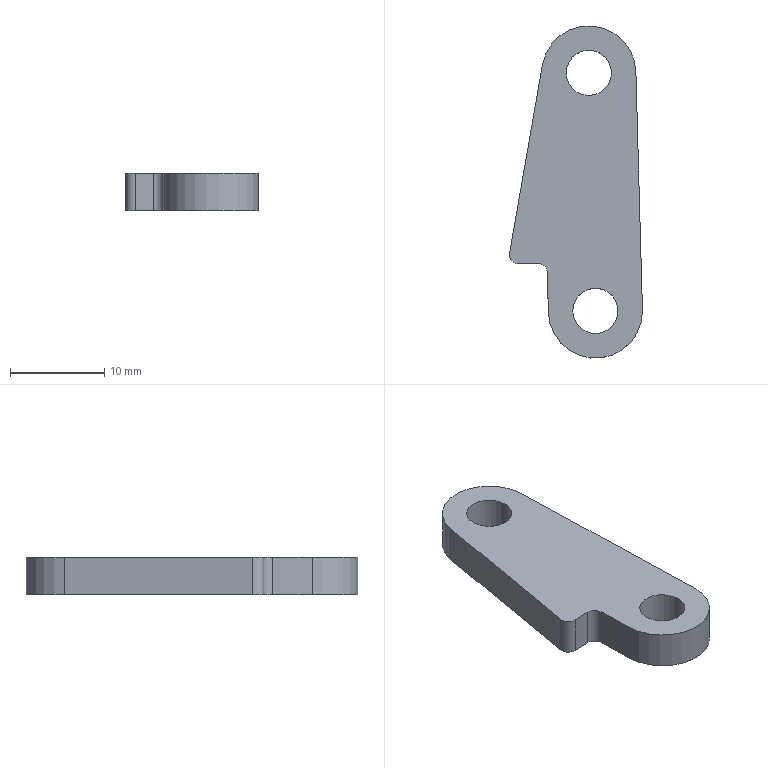Part | SolidWorks | features BaseBody 1 | 1 solid | 15 faces | box 14.127 x 35.318 x 4 mm | volume 1354 mm3 | cylinder 9 | plane 6 | commonest cylinder face diameters 4.8 x4 10 x3 2 x2
STEP:
#1=CARTESIAN_POINT('',(-4.999,-0.1072,-2.));
#2=VERTEX_POINT('',#1);
#3=CARTESIAN_POINT('',(5.,0.,-2.));
#4=VERTEX_POINT('',#3);
#5=CARTESIAN_POINT('',(0.,0.,-2.));
#6=DIRECTION('',(0.,0.,1.));
#7=DIRECTION('',(1.,0.,0.));
#8=AXIS2_PLACEMENT_3D('',#5,#6,#7);
#9=CIRCLE('',#8,5.);
#10=EDGE_CURVE('',#2,#4,#9,.T.);
#11=ORIENTED_EDGE('',*,*,#10,.T.);
#12=CARTESIAN_POINT('',(5.,0.,2.));
#13=VERTEX_POINT('',#12);
#14=CARTESIAN_POINT('',(5.,0.,2.));
#15=DIRECTION('',(0.,0.,1.));
#16=VECTOR('',#15,1000.);
#17=LINE('',#14,#16);
#18=EDGE_CURVE('',#4,#13,#17,.T.);
#19=ORIENTED_EDGE('',*,*,#18,.T.);
#20=CARTESIAN_POINT('',(-4.999,-0.1072,2.));
#21=VERTEX_POINT('',#20);
#22=CARTESIAN_POINT('',(0.,0.,2.));
#23=DIRECTION('',(0.,0.,1.));
#24=DIRECTION('',(1.,0.,0.));
#25=AXIS2_PLACEMENT_3D('',#22,#23,#24);
#26=CIRCLE('',#25,5.);
#27=EDGE_CURVE('',#21,#13,#26,.T.);
#28=ORIENTED_EDGE('',*,*,#27,.F.);
#29=CARTESIAN_POINT('',(-4.999,-0.1072,2.));
#30=DIRECTION('',(0.,0.,-1.));
#31=VECTOR('',#30,1000.);
#32=LINE('',#29,#31);
#33=EDGE_CURVE('',#21,#2,#32,.T.);
#34=ORIENTED_EDGE('',*,*,#33,.T.);
#35=EDGE_LOOP('',(#11,#19,#28,#34));
#36=FACE_OUTER_BOUND('',#35,.T.);
#37=CARTESIAN_POINT('',(0.,0.,2.));
#38=DIRECTION('',(0.,0.,1.));
#39=DIRECTION('',(1.,0.,0.));
#40=AXIS2_PLACEMENT_3D('',#37,#38,#39);
#41=CYLINDRICAL_SURFACE('',#40,5.);
#42=ADVANCED_FACE('',(#36),#41,.T.);
#43=CARTESIAN_POINT('',(-2.401,0.03084,-2.));
#44=VERTEX_POINT('',#43);
#45=CARTESIAN_POINT('',(2.399,0.03084,-2.));
#46=VERTEX_POINT('',#45);
#47=CARTESIAN_POINT('',(-0.0008516,0.03084,-2.));
#48=DIRECTION('',(0.,0.,1.));
#49=DIRECTION('',(1.,0.,0.));
#50=AXIS2_PLACEMENT_3D('',#47,#48,#49);
#51=CIRCLE('',#50,2.4);
#52=EDGE_CURVE('',#44,#46,#51,.T.);
#53=ORIENTED_EDGE('',*,*,#52,.F.);
#54=CARTESIAN_POINT('',(-2.401,0.03084,2.));
#55=VERTEX_POINT('',#54);
#56=CARTESIAN_POINT('',(-2.401,0.03084,2.));
#57=DIRECTION('',(0.,0.,1.));
#58=VECTOR('',#57,1000.);
#59=LINE('',#56,#58);
#60=EDGE_CURVE('',#44,#55,#59,.T.);
#61=ORIENTED_EDGE('',*,*,#60,.T.);
#62=CARTESIAN_POINT('',(2.399,0.03084,2.));
#63=VERTEX_POINT('',#62);
#64=CARTESIAN_POINT('',(-0.0008516,0.03084,2.));
#65=DIRECTION('',(0.,0.,-1.));
#66=DIRECTION('',(1.,0.,0.));
#67=AXIS2_PLACEMENT_3D('',#64,#65,#66);
#68=CIRCLE('',#67,2.4);
#69=EDGE_CURVE('',#63,#55,#68,.T.);
#70=ORIENTED_EDGE('',*,*,#69,.F.);
#71=CARTESIAN_POINT('',(2.399,0.03084,2.));
#72=DIRECTION('',(0.,0.,1.));
#73=VECTOR('',#72,1000.);
#74=LINE('',#71,#73);
#75=EDGE_CURVE('',#46,#63,#74,.T.);
#76=ORIENTED_EDGE('',*,*,#75,.F.);
#77=EDGE_LOOP('',(#53,#61,#70,#76));
#78=FACE_OUTER_BOUND('',#77,.T.);
#79=CARTESIAN_POINT('',(-0.0008516,0.03084,2.));
#80=DIRECTION('',(0.,0.,1.));
#81=DIRECTION('',(1.,0.,0.));
#82=AXIS2_PLACEMENT_3D('',#79,#80,#81);
#83=CYLINDRICAL_SURFACE('',#82,2.4);
#84=ADVANCED_FACE('',(#78),#83,.F.);
#85=CARTESIAN_POINT('',(-3.101,25.331,-2.));
#86=VERTEX_POINT('',#85);
#87=CARTESIAN_POINT('',(1.699,25.331,-2.));
#88=VERTEX_POINT('',#87);
#89=CARTESIAN_POINT('',(-0.7009,25.331,-2.));
#90=DIRECTION('',(0.,0.,1.));
#91=DIRECTION('',(1.,0.,0.));
#92=AXIS2_PLACEMENT_3D('',#89,#90,#91);
#93=CIRCLE('',#92,2.4);
#94=EDGE_CURVE('',#86,#88,#93,.T.);
#95=ORIENTED_EDGE('',*,*,#94,.F.);
#96=CARTESIAN_POINT('',(-3.101,25.331,2.));
#97=VERTEX_POINT('',#96);
#98=CARTESIAN_POINT('',(-3.101,25.331,2.));
#99=DIRECTION('',(0.,0.,1.));
#100=VECTOR('',#99,1000.);
#101=LINE('',#98,#100);
#102=EDGE_CURVE('',#86,#97,#101,.T.);
#103=ORIENTED_EDGE('',*,*,#102,.T.);
#104=CARTESIAN_POINT('',(1.699,25.331,2.));
#105=VERTEX_POINT('',#104);
#106=CARTESIAN_POINT('',(-0.7009,25.331,2.));
#107=DIRECTION('',(0.,0.,-1.));
#108=DIRECTION('',(1.,0.,0.));
#109=AXIS2_PLACEMENT_3D('',#106,#107,#108);
#110=CIRCLE('',#109,2.4);
#111=EDGE_CURVE('',#105,#97,#110,.T.);
#112=ORIENTED_EDGE('',*,*,#111,.F.);
#113=CARTESIAN_POINT('',(1.699,25.331,2.));
#114=DIRECTION('',(0.,0.,1.));
#115=VECTOR('',#114,1000.);
#116=LINE('',#113,#115);
#117=EDGE_CURVE('',#88,#105,#116,.T.);
#118=ORIENTED_EDGE('',*,*,#117,.F.);
#119=EDGE_LOOP('',(#95,#103,#112,#118));
#120=FACE_OUTER_BOUND('',#119,.T.);
#121=CARTESIAN_POINT('',(-0.7009,25.331,2.));
#122=DIRECTION('',(0.,0.,1.));
#123=DIRECTION('',(1.,0.,0.));
#124=AXIS2_PLACEMENT_3D('',#121,#122,#123);
#125=CYLINDRICAL_SURFACE('',#124,2.4);
#126=ADVANCED_FACE('',(#120),#125,.F.);
#127=CARTESIAN_POINT('',(4.997,0.1688,2.));
#128=VERTEX_POINT('',#127);
#129=CARTESIAN_POINT('',(4.299,25.459,2.));
#130=VERTEX_POINT('',#129);
#131=CARTESIAN_POINT('',(4.997,0.1688,2.));
#132=DIRECTION('',(-0.02759,0.9996,0.));
#133=VECTOR('',#132,1000.);
#134=LINE('',#131,#133);
#135=EDGE_CURVE('',#128,#130,#134,.T.);
#136=ORIENTED_EDGE('',*,*,#135,.T.);
#137=CARTESIAN_POINT('',(-5.624,26.181,2.));
#138=VERTEX_POINT('',#137);
#139=CARTESIAN_POINT('',(-0.6989,25.318,2.));
#140=DIRECTION('',(0.,0.,1.));
#141=DIRECTION('',(1.,0.,0.));
#142=AXIS2_PLACEMENT_3D('',#139,#140,#141);
#143=CIRCLE('',#142,5.);
#144=EDGE_CURVE('',#130,#138,#143,.T.);
#145=ORIENTED_EDGE('',*,*,#144,.T.);
#146=CARTESIAN_POINT('',(-9.112,6.191,2.));
#147=VERTEX_POINT('',#146);
#148=CARTESIAN_POINT('',(-5.624,26.181,2.));
#149=DIRECTION('',(-0.1719,-0.9851,0.));
#150=VECTOR('',#149,1000.);
#151=LINE('',#148,#150);
#152=EDGE_CURVE('',#138,#147,#151,.T.);
#153=ORIENTED_EDGE('',*,*,#152,.T.);
#154=CARTESIAN_POINT('',(-8.099,5.02,2.));
#155=VERTEX_POINT('',#154);
#156=CARTESIAN_POINT('',(-8.127,6.019,2.));
#157=DIRECTION('',(0.,0.,1.));
#158=DIRECTION('',(1.,0.,0.));
#159=AXIS2_PLACEMENT_3D('',#156,#157,#158);
#160=CIRCLE('',#159,1.);
#161=EDGE_CURVE('',#147,#155,#160,.T.);
#162=ORIENTED_EDGE('',*,*,#161,.T.);
#163=CARTESIAN_POINT('',(-6.142,5.074,2.));
#164=VERTEX_POINT('',#163);
#165=CARTESIAN_POINT('',(-8.099,5.02,2.));
#166=DIRECTION('',(0.9996,0.0276,0.));
#167=VECTOR('',#166,1000.);
#168=LINE('',#165,#167);
#169=EDGE_CURVE('',#155,#164,#168,.T.);
#170=ORIENTED_EDGE('',*,*,#169,.T.);
#171=CARTESIAN_POINT('',(-5.115,4.102,2.));
#172=VERTEX_POINT('',#171);
#173=CARTESIAN_POINT('',(-6.114,4.074,2.));
#174=DIRECTION('',(0.,0.,-1.));
#175=DIRECTION('',(1.,0.,0.));
#176=AXIS2_PLACEMENT_3D('',#173,#174,#175);
#177=CIRCLE('',#176,1.);
#178=EDGE_CURVE('',#164,#172,#177,.T.);
#179=ORIENTED_EDGE('',*,*,#178,.T.);
#180=CARTESIAN_POINT('',(-5.115,4.102,2.));
#181=DIRECTION('',(0.02755,-0.9996,0.));
#182=VECTOR('',#181,1000.);
#183=LINE('',#180,#182);
#184=EDGE_CURVE('',#172,#21,#183,.T.);
#185=ORIENTED_EDGE('',*,*,#184,.T.);
#186=ORIENTED_EDGE('',*,*,#27,.T.);
#187=CARTESIAN_POINT('',(0.,0.,2.));
#188=DIRECTION('',(0.,0.,1.));
#189=DIRECTION('',(1.,0.,0.));
#190=AXIS2_PLACEMENT_3D('',#187,#188,#189);
#191=CIRCLE('',#190,5.);
#192=EDGE_CURVE('',#13,#128,#191,.T.);
#193=ORIENTED_EDGE('',*,*,#192,.T.);
#194=EDGE_LOOP('',(#136,#145,#153,#162,#170,#179,#185,#186,#193));
#195=FACE_OUTER_BOUND('',#194,.T.);
#196=ORIENTED_EDGE('',*,*,#69,.T.);
#197=CARTESIAN_POINT('',(-0.0008516,0.03084,2.));
#198=DIRECTION('',(0.,0.,-1.));
#199=DIRECTION('',(1.,0.,0.));
#200=AXIS2_PLACEMENT_3D('',#197,#198,#199);
#201=CIRCLE('',#200,2.4);
#202=EDGE_CURVE('',#55,#63,#201,.T.);
#203=ORIENTED_EDGE('',*,*,#202,.T.);
#204=EDGE_LOOP('',(#196,#203));
#205=FACE_BOUND('',#204,.T.);
#206=ORIENTED_EDGE('',*,*,#111,.T.);
#207=CARTESIAN_POINT('',(-0.7009,25.331,2.));
#208=DIRECTION('',(0.,0.,-1.));
#209=DIRECTION('',(1.,0.,0.));
#210=AXIS2_PLACEMENT_3D('',#207,#208,#209);
#211=CIRCLE('',#210,2.4);
#212=EDGE_CURVE('',#97,#105,#211,.T.);
#213=ORIENTED_EDGE('',*,*,#212,.T.);
#214=EDGE_LOOP('',(#206,#213));
#215=FACE_BOUND('',#214,.T.);
#216=CARTESIAN_POINT('',(-8.127,6.019,2.));
#217=DIRECTION('',(0.,0.,1.));
#218=DIRECTION('',(1.,0.,0.));
#219=AXIS2_PLACEMENT_3D('',#216,#217,#218);
#220=PLANE('',#219);
#221=ADVANCED_FACE('',(#195,#205,#215),#220,.T.);
#222=ORIENTED_EDGE('',*,*,#144,.F.);
#223=CARTESIAN_POINT('',(4.299,25.459,-2.));
#224=VERTEX_POINT('',#223);
#225=CARTESIAN_POINT('',(4.299,25.459,2.));
#226=DIRECTION('',(0.,0.,-1.));
#227=VECTOR('',#226,1000.);
#228=LINE('',#225,#227);
#229=EDGE_CURVE('',#130,#224,#228,.T.);
#230=ORIENTED_EDGE('',*,*,#229,.T.);
#231=CARTESIAN_POINT('',(-5.624,26.181,-2.));
#232=VERTEX_POINT('',#231);
#233=CARTESIAN_POINT('',(-0.6989,25.318,-2.));
#234=DIRECTION('',(0.,0.,1.));
#235=DIRECTION('',(1.,0.,0.));
#236=AXIS2_PLACEMENT_3D('',#233,#234,#235);
#237=CIRCLE('',#236,5.);
#238=EDGE_CURVE('',#224,#232,#237,.T.);
#239=ORIENTED_EDGE('',*,*,#238,.T.);
#240=CARTESIAN_POINT('',(-5.624,26.181,2.));
#241=DIRECTION('',(0.,0.,1.));
#242=VECTOR('',#241,1000.);
#243=LINE('',#240,#242);
#244=EDGE_CURVE('',#232,#138,#243,.T.);
#245=ORIENTED_EDGE('',*,*,#244,.T.);
#246=EDGE_LOOP('',(#222,#230,#239,#245));
#247=FACE_OUTER_BOUND('',#246,.T.);
#248=CARTESIAN_POINT('',(-0.6989,25.318,2.));
#249=DIRECTION('',(0.,0.,1.));
#250=DIRECTION('',(1.,0.,0.));
#251=AXIS2_PLACEMENT_3D('',#248,#249,#250);
#252=CYLINDRICAL_SURFACE('',#251,5.);
#253=ADVANCED_FACE('',(#247),#252,.T.);
#254=ORIENTED_EDGE('',*,*,#229,.F.);
#255=ORIENTED_EDGE('',*,*,#135,.F.);
#256=CARTESIAN_POINT('',(4.997,0.1688,-2.));
#257=VERTEX_POINT('',#256);
#258=CARTESIAN_POINT('',(4.997,0.1688,2.));
#259=DIRECTION('',(0.,0.,1.));
#260=VECTOR('',#259,1000.);
#261=LINE('',#258,#260);
#262=EDGE_CURVE('',#257,#128,#261,.T.);
#263=ORIENTED_EDGE('',*,*,#262,.F.);
#264=CARTESIAN_POINT('',(4.997,0.1688,-2.));
#265=DIRECTION('',(0.02759,-0.9996,0.));
#266=VECTOR('',#265,1000.);
#267=LINE('',#264,#266);
#268=EDGE_CURVE('',#224,#257,#267,.T.);
#269=ORIENTED_EDGE('',*,*,#268,.F.);
#270=EDGE_LOOP('',(#254,#255,#263,#269));
#271=FACE_OUTER_BOUND('',#270,.T.);
#272=CARTESIAN_POINT('',(4.997,0.1688,2.));
#273=DIRECTION('',(-0.9996,-0.02759,0.));
#274=DIRECTION('',(0.02759,-0.9996,0.));
#275=AXIS2_PLACEMENT_3D('',#272,#273,#274);
#276=PLANE('',#275);
#277=ADVANCED_FACE('',(#271),#276,.F.);
#278=ORIENTED_EDGE('',*,*,#18,.F.);
#279=CARTESIAN_POINT('',(0.,0.,-2.));
#280=DIRECTION('',(0.,0.,1.));
#281=DIRECTION('',(1.,0.,0.));
#282=AXIS2_PLACEMENT_3D('',#279,#280,#281);
#283=CIRCLE('',#282,5.);
#284=EDGE_CURVE('',#4,#257,#283,.T.);
#285=ORIENTED_EDGE('',*,*,#284,.T.);
#286=ORIENTED_EDGE('',*,*,#262,.T.);
#287=ORIENTED_EDGE('',*,*,#192,.F.);
#288=EDGE_LOOP('',(#278,#285,#286,#287));
#289=FACE_OUTER_BOUND('',#288,.T.);
#290=CARTESIAN_POINT('',(0.,0.,2.));
#291=DIRECTION('',(0.,0.,1.));
#292=DIRECTION('',(1.,0.,0.));
#293=AXIS2_PLACEMENT_3D('',#290,#291,#292);
#294=CYLINDRICAL_SURFACE('',#293,5.);
#295=ADVANCED_FACE('',(#289),#294,.T.);
#296=ORIENTED_EDGE('',*,*,#33,.F.);
#297=ORIENTED_EDGE('',*,*,#184,.F.);
#298=CARTESIAN_POINT('',(-5.115,4.102,-2.));
#299=VERTEX_POINT('',#298);
#300=CARTESIAN_POINT('',(-5.115,4.102,2.));
#301=DIRECTION('',(0.,0.,1.));
#302=VECTOR('',#301,1000.);
#303=LINE('',#300,#302);
#304=EDGE_CURVE('',#299,#172,#303,.T.);
#305=ORIENTED_EDGE('',*,*,#304,.F.);
#306=CARTESIAN_POINT('',(-5.115,4.102,-2.));
#307=DIRECTION('',(-0.02755,0.9996,0.));
#308=VECTOR('',#307,1000.);
#309=LINE('',#306,#308);
#310=EDGE_CURVE('',#2,#299,#309,.T.);
#311=ORIENTED_EDGE('',*,*,#310,.F.);
#312=EDGE_LOOP('',(#296,#297,#305,#311));
#313=FACE_OUTER_BOUND('',#312,.T.);
#314=CARTESIAN_POINT('',(-5.115,4.102,2.));
#315=DIRECTION('',(0.9996,0.02755,0.));
#316=DIRECTION('',(-0.02755,0.9996,0.));
#317=AXIS2_PLACEMENT_3D('',#314,#315,#316);
#318=PLANE('',#317);
#319=ADVANCED_FACE('',(#313),#318,.F.);
#320=CARTESIAN_POINT('',(-6.142,5.074,-2.));
#321=VERTEX_POINT('',#320);
#322=CARTESIAN_POINT('',(-6.142,5.074,2.));
#323=DIRECTION('',(0.,0.,-1.));
#324=VECTOR('',#323,1000.);
#325=LINE('',#322,#324);
#326=EDGE_CURVE('',#164,#321,#325,.T.);
#327=ORIENTED_EDGE('',*,*,#326,.F.);
#328=ORIENTED_EDGE('',*,*,#169,.F.);
#329=CARTESIAN_POINT('',(-8.099,5.02,-2.));
#330=VERTEX_POINT('',#329);
#331=CARTESIAN_POINT('',(-8.099,5.02,2.));
#332=DIRECTION('',(0.,0.,1.));
#333=VECTOR('',#332,1000.);
#334=LINE('',#331,#333);
#335=EDGE_CURVE('',#330,#155,#334,.T.);
#336=ORIENTED_EDGE('',*,*,#335,.F.);
#337=CARTESIAN_POINT('',(-8.099,5.02,-2.));
#338=DIRECTION('',(-0.9996,-0.0276,0.));
#339=VECTOR('',#338,1000.);
#340=LINE('',#337,#339);
#341=EDGE_CURVE('',#321,#330,#340,.T.);
#342=ORIENTED_EDGE('',*,*,#341,.F.);
#343=EDGE_LOOP('',(#327,#328,#336,#342));
#344=FACE_OUTER_BOUND('',#343,.T.);
#345=CARTESIAN_POINT('',(-8.099,5.02,2.));
#346=DIRECTION('',(-0.0276,0.9996,0.));
#347=DIRECTION('',(-0.9996,-0.0276,0.));
#348=AXIS2_PLACEMENT_3D('',#345,#346,#347);
#349=PLANE('',#348);
#350=ADVANCED_FACE('',(#344),#349,.F.);
#351=ORIENTED_EDGE('',*,*,#161,.F.);
#352=CARTESIAN_POINT('',(-9.112,6.191,-2.));
#353=VERTEX_POINT('',#352);
#354=CARTESIAN_POINT('',(-9.112,6.191,2.));
#355=DIRECTION('',(0.,0.,-1.));
#356=VECTOR('',#355,1000.);
#357=LINE('',#354,#356);
#358=EDGE_CURVE('',#147,#353,#357,.T.);
#359=ORIENTED_EDGE('',*,*,#358,.T.);
#360=CARTESIAN_POINT('',(-8.127,6.019,-2.));
#361=DIRECTION('',(0.,0.,1.));
#362=DIRECTION('',(1.,0.,0.));
#363=AXIS2_PLACEMENT_3D('',#360,#361,#362);
#364=CIRCLE('',#363,1.);
#365=EDGE_CURVE('',#353,#330,#364,.T.);
#366=ORIENTED_EDGE('',*,*,#365,.T.);
#367=ORIENTED_EDGE('',*,*,#335,.T.);
#368=EDGE_LOOP('',(#351,#359,#366,#367));
#369=FACE_OUTER_BOUND('',#368,.T.);
#370=CARTESIAN_POINT('',(-8.127,6.019,2.));
#371=DIRECTION('',(0.,0.,1.));
#372=DIRECTION('',(1.,0.,0.));
#373=AXIS2_PLACEMENT_3D('',#370,#371,#372);
#374=CYLINDRICAL_SURFACE('',#373,1.);
#375=ADVANCED_FACE('',(#369),#374,.T.);
#376=ORIENTED_EDGE('',*,*,#358,.F.);
#377=ORIENTED_EDGE('',*,*,#152,.F.);
#378=ORIENTED_EDGE('',*,*,#244,.F.);
#379=CARTESIAN_POINT('',(-5.624,26.181,-2.));
#380=DIRECTION('',(0.1719,0.9851,0.));
#381=VECTOR('',#380,1000.);
#382=LINE('',#379,#381);
#383=EDGE_CURVE('',#353,#232,#382,.T.);
#384=ORIENTED_EDGE('',*,*,#383,.F.);
#385=EDGE_LOOP('',(#376,#377,#378,#384));
#386=FACE_OUTER_BOUND('',#385,.T.);
#387=CARTESIAN_POINT('',(-5.624,26.181,2.));
#388=DIRECTION('',(0.9851,-0.1719,0.));
#389=DIRECTION('',(0.1719,0.9851,0.));
#390=AXIS2_PLACEMENT_3D('',#387,#388,#389);
#391=PLANE('',#390);
#392=ADVANCED_FACE('',(#386),#391,.F.);
#393=ORIENTED_EDGE('',*,*,#60,.F.);
#394=CARTESIAN_POINT('',(-0.0008516,0.03084,-2.));
#395=DIRECTION('',(0.,0.,1.));
#396=DIRECTION('',(1.,0.,0.));
#397=AXIS2_PLACEMENT_3D('',#394,#395,#396);
#398=CIRCLE('',#397,2.4);
#399=EDGE_CURVE('',#46,#44,#398,.T.);
#400=ORIENTED_EDGE('',*,*,#399,.F.);
#401=ORIENTED_EDGE('',*,*,#75,.T.);
#402=ORIENTED_EDGE('',*,*,#202,.F.);
#403=EDGE_LOOP('',(#393,#400,#401,#402));
#404=FACE_OUTER_BOUND('',#403,.T.);
#405=CARTESIAN_POINT('',(-0.0008516,0.03084,2.));
#406=DIRECTION('',(0.,0.,1.));
#407=DIRECTION('',(1.,0.,0.));
#408=AXIS2_PLACEMENT_3D('',#405,#406,#407);
#409=CYLINDRICAL_SURFACE('',#408,2.4);
#410=ADVANCED_FACE('',(#404),#409,.F.);
#411=ORIENTED_EDGE('',*,*,#102,.F.);
#412=CARTESIAN_POINT('',(-0.7009,25.331,-2.));
#413=DIRECTION('',(0.,0.,1.));
#414=DIRECTION('',(1.,0.,0.));
#415=AXIS2_PLACEMENT_3D('',#412,#413,#414);
#416=CIRCLE('',#415,2.4);
#417=EDGE_CURVE('',#88,#86,#416,.T.);
#418=ORIENTED_EDGE('',*,*,#417,.F.);
#419=ORIENTED_EDGE('',*,*,#117,.T.);
#420=ORIENTED_EDGE('',*,*,#212,.F.);
#421=EDGE_LOOP('',(#411,#418,#419,#420));
#422=FACE_OUTER_BOUND('',#421,.T.);
#423=CARTESIAN_POINT('',(-0.7009,25.331,2.));
#424=DIRECTION('',(0.,0.,1.));
#425=DIRECTION('',(1.,0.,0.));
#426=AXIS2_PLACEMENT_3D('',#423,#424,#425);
#427=CYLINDRICAL_SURFACE('',#426,2.4);
#428=ADVANCED_FACE('',(#422),#427,.F.);
#429=ORIENTED_EDGE('',*,*,#238,.F.);
#430=ORIENTED_EDGE('',*,*,#268,.T.);
#431=ORIENTED_EDGE('',*,*,#284,.F.);
#432=ORIENTED_EDGE('',*,*,#10,.F.);
#433=ORIENTED_EDGE('',*,*,#310,.T.);
#434=CARTESIAN_POINT('',(-6.114,4.074,-2.));
#435=DIRECTION('',(0.,0.,-1.));
#436=DIRECTION('',(1.,0.,0.));
#437=AXIS2_PLACEMENT_3D('',#434,#435,#436);
#438=CIRCLE('',#437,1.);
#439=EDGE_CURVE('',#321,#299,#438,.T.);
#440=ORIENTED_EDGE('',*,*,#439,.F.);
#441=ORIENTED_EDGE('',*,*,#341,.T.);
#442=ORIENTED_EDGE('',*,*,#365,.F.);
#443=ORIENTED_EDGE('',*,*,#383,.T.);
#444=EDGE_LOOP('',(#429,#430,#431,#432,#433,#440,#441,#442,#443));
#445=FACE_OUTER_BOUND('',#444,.T.);
#446=ORIENTED_EDGE('',*,*,#399,.T.);
#447=ORIENTED_EDGE('',*,*,#52,.T.);
#448=EDGE_LOOP('',(#446,#447));
#449=FACE_BOUND('',#448,.T.);
#450=ORIENTED_EDGE('',*,*,#417,.T.);
#451=ORIENTED_EDGE('',*,*,#94,.T.);
#452=EDGE_LOOP('',(#450,#451));
#453=FACE_BOUND('',#452,.T.);
#454=CARTESIAN_POINT('',(-8.127,6.019,-2.));
#455=DIRECTION('',(0.,0.,1.));
#456=DIRECTION('',(1.,0.,0.));
#457=AXIS2_PLACEMENT_3D('',#454,#455,#456);
#458=PLANE('',#457);
#459=ADVANCED_FACE('',(#445,#449,#453),#458,.F.);
#460=ORIENTED_EDGE('',*,*,#304,.T.);
#461=ORIENTED_EDGE('',*,*,#178,.F.);
#462=ORIENTED_EDGE('',*,*,#326,.T.);
#463=ORIENTED_EDGE('',*,*,#439,.T.);
#464=EDGE_LOOP('',(#460,#461,#462,#463));
#465=FACE_OUTER_BOUND('',#464,.T.);
#466=CARTESIAN_POINT('',(-6.114,4.074,2.));
#467=DIRECTION('',(0.,0.,1.));
#468=DIRECTION('',(1.,0.,0.));
#469=AXIS2_PLACEMENT_3D('',#466,#467,#468);
#470=CYLINDRICAL_SURFACE('',#469,1.);
#471=ADVANCED_FACE('',(#465),#470,.F.);
#472=CLOSED_SHELL('',(#42,#84,#126,#221,#253,#277,#295,#319,#350,#375,#392,#410,#428,#459,#471));
#473=MANIFOLD_SOLID_BREP('',#472);
#474=CARTESIAN_POINT('',(0.,0.,0.));
#475=DIRECTION('',(0.,0.,1.));
#476=DIRECTION('',(1.,0.,0.));
#477=AXIS2_PLACEMENT_3D('',#474,#475,#476);
#478=(LENGTH_UNIT()NAMED_UNIT(*)SI_UNIT(.MILLI.,.METRE.));
#479=UNCERTAINTY_MEASURE_WITH_UNIT(LENGTH_MEASURE(0.00001),#478,'','');
#480=(NAMED_UNIT(*)PLANE_ANGLE_UNIT()SI_UNIT($,.RADIAN.));
#481=(NAMED_UNIT(*)SI_UNIT($,.STERADIAN.)SOLID_ANGLE_UNIT());
#482=(GEOMETRIC_REPRESENTATION_CONTEXT(3)GLOBAL_UNCERTAINTY_ASSIGNED_CONTEXT((#479))GLOBAL_UNIT_ASSIGNED_CONTEXT((#478,#480,#481))REPRESENTATION_CONTEXT('',''));
#483=ADVANCED_BREP_SHAPE_REPRESENTATION('',(#473,#477),#482);